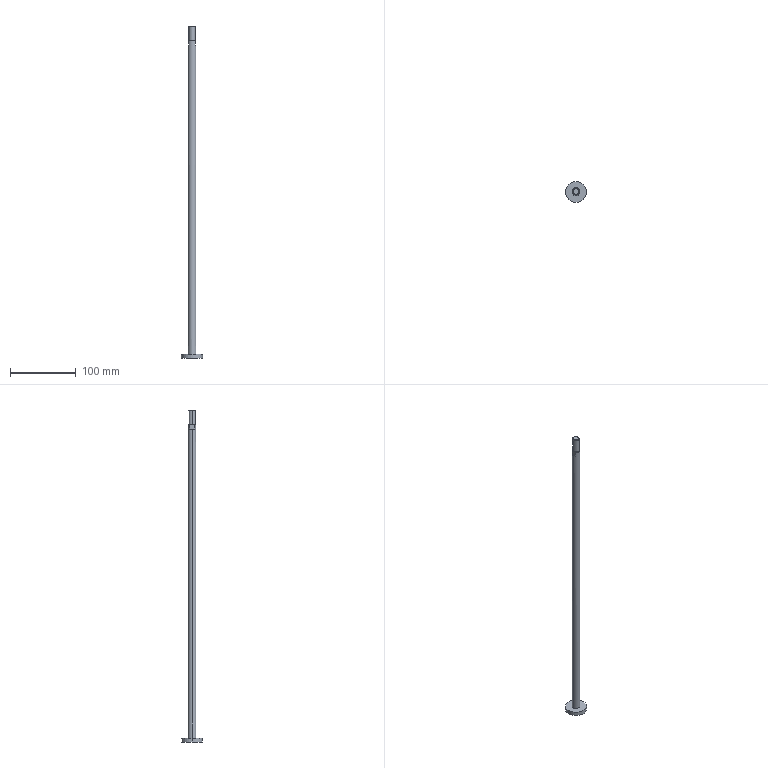Part | STEP file | 1 solid | 17 faces | box 32 x 32 x 503.2 mm | volume 60225 mm3 | plane 9 | cylinder 6 | cone 2 | commonest cylinder face diameters 10 x2 12 x2 32 x2
STEP:
#1=CARTESIAN_POINT('',(0.,0.,0.));
#2=DIRECTION('',(0.,0.,1.));
#3=DIRECTION('',(1.,0.,0.));
#4=AXIS2_PLACEMENT_3D('',#1,#2,#3);
#5=CARTESIAN_POINT('',(5.,0.,26.));
#6=VERTEX_POINT('',#5);
#7=CARTESIAN_POINT('',(-5.,0.,26.));
#8=VERTEX_POINT('',#7);
#9=CARTESIAN_POINT('',(0.,0.,26.));
#10=DIRECTION('',(0.,0.,1.));
#11=DIRECTION('',(1.,0.,0.));
#12=AXIS2_PLACEMENT_3D('',#9,#10,#11);
#13=CIRCLE('',#12,5.);
#14=CARTESIAN_POINT('',(0.,0.,26.));
#15=DIRECTION('',(0.,0.,1.));
#16=DIRECTION('',(1.,0.,0.));
#17=AXIS2_PLACEMENT_3D('',#14,#15,#16);
#18=CYLINDRICAL_SURFACE('',#17,5.);
#19=CARTESIAN_POINT('',(0.,0.));
#20=DIRECTION('',(1.,0.));
#21=VECTOR('',#20,1.);
#22=LINE('',#19,#21);
#23=(GEOMETRIC_REPRESENTATION_CONTEXT(2)PARAMETRIC_REPRESENTATION_CONTEXT()REPRESENTATION_CONTEXT('',''));
#24=DEFINITIONAL_REPRESENTATION('',(#22),#23);
#25=PCURVE('',#18,#24);
#26=CARTESIAN_POINT('',(0.,0.,26.));
#27=DIRECTION('',(0.,0.,-1.));
#28=DIRECTION('',(-1.,0.,0.));
#29=AXIS2_PLACEMENT_3D('',#26,#27,#28);
#30=PLANE('',#29);
#31=CARTESIAN_POINT('',(-5.,0.));
#32=CARTESIAN_POINT('',(-5.,8.66));
#33=CARTESIAN_POINT('',(2.5,4.33));
#34=CARTESIAN_POINT('',(10.,0.));
#35=CARTESIAN_POINT('',(2.5,-4.33));
#36=CARTESIAN_POINT('',(-5.,-8.66));
#37=CARTESIAN_POINT('',(-5.,0.));
#38=(BOUNDED_CURVE()B_SPLINE_CURVE(2,(#31,#32,#33,#34,#35,#36,#37),.UNSPECIFIED.,.T.,.F.)B_SPLINE_CURVE_WITH_KNOTS((1,2,2,2,2,1),(-2.094,0.,2.094,4.189,6.283,8.378),.UNSPECIFIED.)CURVE()GEOMETRIC_REPRESENTATION_ITEM()RATIONAL_B_SPLINE_CURVE((1.,0.5,1.,0.5,1.,0.5,1.))REPRESENTATION_ITEM(''));
#39=(GEOMETRIC_REPRESENTATION_CONTEXT(2)PARAMETRIC_REPRESENTATION_CONTEXT()REPRESENTATION_CONTEXT('',''));
#40=DEFINITIONAL_REPRESENTATION('',(#38),#39);
#41=PCURVE('',#30,#40);
#42=SURFACE_CURVE('',#13,(#25,#41),.PCURVE_S1.);
#43=EDGE_CURVE('',#6,#8,#42,.T.);
#44=ORIENTED_EDGE('',*,*,#43,.T.);
#45=CARTESIAN_POINT('',(-5.,0.,47.233));
#46=VERTEX_POINT('',#45);
#47=CARTESIAN_POINT('',(-5.,0.,26.));
#48=DIRECTION('',(0.,0.,1.));
#49=VECTOR('',#48,1.);
#50=LINE('',#47,#49);
#51=CARTESIAN_POINT('',(3.142,0.));
#52=DIRECTION('',(0.,1.));
#53=VECTOR('',#52,1.);
#54=LINE('',#51,#53);
#55=(GEOMETRIC_REPRESENTATION_CONTEXT(2)PARAMETRIC_REPRESENTATION_CONTEXT()REPRESENTATION_CONTEXT('',''));
#56=DEFINITIONAL_REPRESENTATION('',(#54),#55);
#57=PCURVE('',#18,#56);
#58=CARTESIAN_POINT('',(0.,0.,26.));
#59=DIRECTION('',(0.,0.,1.));
#60=DIRECTION('',(1.,0.,0.));
#61=AXIS2_PLACEMENT_3D('',#58,#59,#60);
#62=CYLINDRICAL_SURFACE('',#61,5.);
#63=CARTESIAN_POINT('',(3.142,0.));
#64=DIRECTION('',(0.,1.));
#65=VECTOR('',#64,1.);
#66=LINE('',#63,#65);
#67=(GEOMETRIC_REPRESENTATION_CONTEXT(2)PARAMETRIC_REPRESENTATION_CONTEXT()REPRESENTATION_CONTEXT('',''));
#68=DEFINITIONAL_REPRESENTATION('',(#66),#67);
#69=PCURVE('',#62,#68);
#70=SURFACE_CURVE('',#50,(#57,#69),.PCURVE_S1.);
#71=EDGE_CURVE('',#8,#46,#70,.T.);
#72=ORIENTED_EDGE('',*,*,#71,.T.);
#73=CARTESIAN_POINT('',(5.,0.,47.233));
#74=VERTEX_POINT('',#73);
#75=CARTESIAN_POINT('',(0.,0.,47.233));
#76=DIRECTION('',(0.,0.,1.));
#77=DIRECTION('',(1.,0.,0.));
#78=AXIS2_PLACEMENT_3D('',#75,#76,#77);
#79=CIRCLE('',#78,5.);
#80=CARTESIAN_POINT('',(0.,21.233));
#81=DIRECTION('',(1.,0.));
#82=VECTOR('',#81,1.);
#83=LINE('',#80,#82);
#84=(GEOMETRIC_REPRESENTATION_CONTEXT(2)PARAMETRIC_REPRESENTATION_CONTEXT()REPRESENTATION_CONTEXT('',''));
#85=DEFINITIONAL_REPRESENTATION('',(#83),#84);
#86=PCURVE('',#18,#85);
#87=CARTESIAN_POINT('',(0.,0.,47.233));
#88=DIRECTION('',(0.,0.,-1.));
#89=DIRECTION('',(-1.,0.,0.));
#90=AXIS2_PLACEMENT_3D('',#87,#88,#89);
#91=CONICAL_SURFACE('',#90,5.,0.7854);
#92=CARTESIAN_POINT('',(3.142,0.));
#93=DIRECTION('',(-1.,0.));
#94=VECTOR('',#93,1.);
#95=LINE('',#92,#94);
#96=(GEOMETRIC_REPRESENTATION_CONTEXT(2)PARAMETRIC_REPRESENTATION_CONTEXT()REPRESENTATION_CONTEXT('',''));
#97=DEFINITIONAL_REPRESENTATION('',(#95),#96);
#98=PCURVE('',#91,#97);
#99=SURFACE_CURVE('',#79,(#86,#98),.PCURVE_S1.);
#100=EDGE_CURVE('',#74,#46,#99,.T.);
#101=ORIENTED_EDGE('',*,*,#100,.F.);
#102=CARTESIAN_POINT('',(5.,0.,26.));
#103=DIRECTION('',(0.,0.,1.));
#104=VECTOR('',#103,1.);
#105=LINE('',#102,#104);
#106=CARTESIAN_POINT('',(0.,0.));
#107=DIRECTION('',(0.,1.));
#108=VECTOR('',#107,1.);
#109=LINE('',#106,#108);
#110=(GEOMETRIC_REPRESENTATION_CONTEXT(2)PARAMETRIC_REPRESENTATION_CONTEXT()REPRESENTATION_CONTEXT('',''));
#111=DEFINITIONAL_REPRESENTATION('',(#109),#110);
#112=PCURVE('',#18,#111);
#113=CARTESIAN_POINT('',(6.283,0.));
#114=DIRECTION('',(0.,1.));
#115=VECTOR('',#114,1.);
#116=LINE('',#113,#115);
#117=(GEOMETRIC_REPRESENTATION_CONTEXT(2)PARAMETRIC_REPRESENTATION_CONTEXT()REPRESENTATION_CONTEXT('',''));
#118=DEFINITIONAL_REPRESENTATION('',(#116),#117);
#119=PCURVE('',#62,#118);
#120=SURFACE_CURVE('',#105,(#112,#119),.PCURVE_S1.);
#121=EDGE_CURVE('',#6,#74,#120,.T.);
#122=ORIENTED_EDGE('',*,*,#121,.F.);
#123=EDGE_LOOP('',(#44,#72,#101,#122));
#124=FACE_BOUND('',#123,.T.);
#125=ADVANCED_FACE('',(#124),#18,.T.);
#126=CARTESIAN_POINT('',(4.233,0.,48.));
#127=VERTEX_POINT('',#126);
#128=CARTESIAN_POINT('',(-4.233,0.,48.));
#129=VERTEX_POINT('',#128);
#130=CARTESIAN_POINT('',(0.,0.,48.));
#131=DIRECTION('',(0.,0.,1.));
#132=DIRECTION('',(1.,0.,0.));
#133=AXIS2_PLACEMENT_3D('',#130,#131,#132);
#134=CIRCLE('',#133,4.233);
#135=CARTESIAN_POINT('',(3.142,-0.767));
#136=DIRECTION('',(-1.,0.));
#137=VECTOR('',#136,1.);
#138=LINE('',#135,#137);
#139=(GEOMETRIC_REPRESENTATION_CONTEXT(2)PARAMETRIC_REPRESENTATION_CONTEXT()REPRESENTATION_CONTEXT('',''));
#140=DEFINITIONAL_REPRESENTATION('',(#138),#139);
#141=PCURVE('',#91,#140);
#142=CARTESIAN_POINT('',(0.,0.,48.));
#143=DIRECTION('',(0.,0.,-1.));
#144=DIRECTION('',(-1.,0.,0.));
#145=AXIS2_PLACEMENT_3D('',#142,#143,#144);
#146=PLANE('',#145);
#147=CARTESIAN_POINT('',(-4.233,0.));
#148=CARTESIAN_POINT('',(-4.233,7.332));
#149=CARTESIAN_POINT('',(2.116,3.666));
#150=CARTESIAN_POINT('',(8.466,0.));
#151=CARTESIAN_POINT('',(2.116,-3.666));
#152=CARTESIAN_POINT('',(-4.233,-7.332));
#153=CARTESIAN_POINT('',(-4.233,0.));
#154=(BOUNDED_CURVE()B_SPLINE_CURVE(2,(#147,#148,#149,#150,#151,#152,#153),.UNSPECIFIED.,.T.,.F.)B_SPLINE_CURVE_WITH_KNOTS((1,2,2,2,2,1),(-2.094,0.,2.094,4.189,6.283,8.378),.UNSPECIFIED.)CURVE()GEOMETRIC_REPRESENTATION_ITEM()RATIONAL_B_SPLINE_CURVE((1.,0.5,1.,0.5,1.,0.5,1.))REPRESENTATION_ITEM(''));
#155=(GEOMETRIC_REPRESENTATION_CONTEXT(2)PARAMETRIC_REPRESENTATION_CONTEXT()REPRESENTATION_CONTEXT('',''));
#156=DEFINITIONAL_REPRESENTATION('',(#154),#155);
#157=PCURVE('',#146,#156);
#158=SURFACE_CURVE('',#134,(#141,#157),.PCURVE_S1.);
#159=EDGE_CURVE('',#127,#129,#158,.T.);
#160=ORIENTED_EDGE('',*,*,#159,.F.);
#161=CARTESIAN_POINT('',(5.,0.,47.233));
#162=DIRECTION('',(0.7071,0.,-0.7071));
#163=VECTOR('',#162,1.);
#164=LINE('',#161,#163);
#165=CARTESIAN_POINT('',(3.142,0.));
#166=DIRECTION('',(0.,1.));
#167=VECTOR('',#166,1.);
#168=LINE('',#165,#167);
#169=(GEOMETRIC_REPRESENTATION_CONTEXT(2)PARAMETRIC_REPRESENTATION_CONTEXT()REPRESENTATION_CONTEXT('',''));
#170=DEFINITIONAL_REPRESENTATION('',(#168),#169);
#171=PCURVE('',#91,#170);
#172=CARTESIAN_POINT('',(0.,0.,47.233));
#173=DIRECTION('',(0.,0.,-1.));
#174=DIRECTION('',(-1.,0.,0.));
#175=AXIS2_PLACEMENT_3D('',#172,#173,#174);
#176=CONICAL_SURFACE('',#175,5.,0.7854);
#177=CARTESIAN_POINT('',(3.142,0.));
#178=DIRECTION('',(0.,1.));
#179=VECTOR('',#178,1.);
#180=LINE('',#177,#179);
#181=(GEOMETRIC_REPRESENTATION_CONTEXT(2)PARAMETRIC_REPRESENTATION_CONTEXT()REPRESENTATION_CONTEXT('',''));
#182=DEFINITIONAL_REPRESENTATION('',(#180),#181);
#183=PCURVE('',#176,#182);
#184=SURFACE_CURVE('',#164,(#171,#183),.PCURVE_S1.);
#185=EDGE_CURVE('',#127,#74,#184,.T.);
#186=ORIENTED_EDGE('',*,*,#185,.T.);
#187=ORIENTED_EDGE('',*,*,#100,.T.);
#188=CARTESIAN_POINT('',(-5.,0.,47.233));
#189=DIRECTION('',(-0.7071,0.,-0.7071));
#190=VECTOR('',#189,1.);
#191=LINE('',#188,#190);
#192=CARTESIAN_POINT('',(0.,0.));
#193=DIRECTION('',(0.,1.));
#194=VECTOR('',#193,1.);
#195=LINE('',#192,#194);
#196=(GEOMETRIC_REPRESENTATION_CONTEXT(2)PARAMETRIC_REPRESENTATION_CONTEXT()REPRESENTATION_CONTEXT('',''));
#197=DEFINITIONAL_REPRESENTATION('',(#195),#196);
#198=PCURVE('',#91,#197);
#199=CARTESIAN_POINT('',(6.283,0.));
#200=DIRECTION('',(0.,1.));
#201=VECTOR('',#200,1.);
#202=LINE('',#199,#201);
#203=(GEOMETRIC_REPRESENTATION_CONTEXT(2)PARAMETRIC_REPRESENTATION_CONTEXT()REPRESENTATION_CONTEXT('',''));
#204=DEFINITIONAL_REPRESENTATION('',(#202),#203);
#205=PCURVE('',#176,#204);
#206=SURFACE_CURVE('',#191,(#198,#205),.PCURVE_S1.);
#207=EDGE_CURVE('',#129,#46,#206,.T.);
#208=ORIENTED_EDGE('',*,*,#207,.F.);
#209=EDGE_LOOP('',(#160,#186,#187,#208));
#210=FACE_BOUND('',#209,.T.);
#211=ADVANCED_FACE('',(#210),#91,.T.);
#212=CARTESIAN_POINT('',(16.,0.,-455.2));
#213=VERTEX_POINT('',#212);
#214=CARTESIAN_POINT('',(-16.,0.,-455.2));
#215=VERTEX_POINT('',#214);
#216=CARTESIAN_POINT('',(0.,0.,-455.2));
#217=DIRECTION('',(0.,0.,1.));
#218=DIRECTION('',(1.,0.,0.));
#219=AXIS2_PLACEMENT_3D('',#216,#217,#218);
#220=CIRCLE('',#219,16.);
#221=CARTESIAN_POINT('',(0.,0.,-455.2));
#222=DIRECTION('',(0.,0.,1.));
#223=DIRECTION('',(1.,0.,0.));
#224=AXIS2_PLACEMENT_3D('',#221,#222,#223);
#225=CYLINDRICAL_SURFACE('',#224,16.);
#226=CARTESIAN_POINT('',(0.,0.));
#227=DIRECTION('',(1.,0.));
#228=VECTOR('',#227,1.);
#229=LINE('',#226,#228);
#230=(GEOMETRIC_REPRESENTATION_CONTEXT(2)PARAMETRIC_REPRESENTATION_CONTEXT()REPRESENTATION_CONTEXT('',''));
#231=DEFINITIONAL_REPRESENTATION('',(#229),#230);
#232=PCURVE('',#225,#231);
#233=CARTESIAN_POINT('',(0.,16.,-455.2));
#234=DIRECTION('',(0.,0.,1.));
#235=DIRECTION('',(1.,0.,0.));
#236=AXIS2_PLACEMENT_3D('',#233,#234,#235);
#237=PLANE('',#236);
#238=CARTESIAN_POINT('',(0.,-16.));
#239=DIRECTION('',(1.,0.));
#240=AXIS2_PLACEMENT_2D('',#238,#239);
#241=CIRCLE('',#240,16.);
#242=(GEOMETRIC_REPRESENTATION_CONTEXT(2)PARAMETRIC_REPRESENTATION_CONTEXT()REPRESENTATION_CONTEXT('',''));
#243=DEFINITIONAL_REPRESENTATION('',(#241),#242);
#244=PCURVE('',#237,#243);
#245=SURFACE_CURVE('',#220,(#232,#244),.PCURVE_S1.);
#246=EDGE_CURVE('',#213,#215,#245,.T.);
#247=ORIENTED_EDGE('',*,*,#246,.T.);
#248=CARTESIAN_POINT('',(-16.,0.,-449.2));
#249=VERTEX_POINT('',#248);
#250=CARTESIAN_POINT('',(-16.,0.,-455.2));
#251=DIRECTION('',(0.,0.,1.));
#252=VECTOR('',#251,1.);
#253=LINE('',#250,#252);
#254=CARTESIAN_POINT('',(3.142,0.));
#255=DIRECTION('',(0.,1.));
#256=VECTOR('',#255,1.);
#257=LINE('',#254,#256);
#258=(GEOMETRIC_REPRESENTATION_CONTEXT(2)PARAMETRIC_REPRESENTATION_CONTEXT()REPRESENTATION_CONTEXT('',''));
#259=DEFINITIONAL_REPRESENTATION('',(#257),#258);
#260=PCURVE('',#225,#259);
#261=CARTESIAN_POINT('',(0.,0.,-455.2));
#262=DIRECTION('',(0.,0.,1.));
#263=DIRECTION('',(1.,0.,0.));
#264=AXIS2_PLACEMENT_3D('',#261,#262,#263);
#265=CYLINDRICAL_SURFACE('',#264,16.);
#266=CARTESIAN_POINT('',(3.142,0.));
#267=DIRECTION('',(0.,1.));
#268=VECTOR('',#267,1.);
#269=LINE('',#266,#268);
#270=(GEOMETRIC_REPRESENTATION_CONTEXT(2)PARAMETRIC_REPRESENTATION_CONTEXT()REPRESENTATION_CONTEXT('',''));
#271=DEFINITIONAL_REPRESENTATION('',(#269),#270);
#272=PCURVE('',#265,#271);
#273=SURFACE_CURVE('',#253,(#260,#272),.PCURVE_S1.);
#274=EDGE_CURVE('',#215,#249,#273,.T.);
#275=ORIENTED_EDGE('',*,*,#274,.T.);
#276=CARTESIAN_POINT('',(16.,0.,-449.2));
#277=VERTEX_POINT('',#276);
#278=CARTESIAN_POINT('',(0.,0.,-449.2));
#279=DIRECTION('',(0.,0.,1.));
#280=DIRECTION('',(1.,0.,0.));
#281=AXIS2_PLACEMENT_3D('',#278,#279,#280);
#282=CIRCLE('',#281,16.);
#283=CARTESIAN_POINT('',(0.,6.));
#284=DIRECTION('',(1.,0.));
#285=VECTOR('',#284,1.);
#286=LINE('',#283,#285);
#287=(GEOMETRIC_REPRESENTATION_CONTEXT(2)PARAMETRIC_REPRESENTATION_CONTEXT()REPRESENTATION_CONTEXT('',''));
#288=DEFINITIONAL_REPRESENTATION('',(#286),#287);
#289=PCURVE('',#225,#288);
#290=CARTESIAN_POINT('',(0.,6.,-449.2));
#291=DIRECTION('',(0.,0.,-1.));
#292=DIRECTION('',(-1.,0.,0.));
#293=AXIS2_PLACEMENT_3D('',#290,#291,#292);
#294=PLANE('',#293);
#295=CARTESIAN_POINT('',(-16.,-6.));
#296=CARTESIAN_POINT('',(-16.,21.713));
#297=CARTESIAN_POINT('',(8.,7.856));
#298=CARTESIAN_POINT('',(32.,-6.));
#299=CARTESIAN_POINT('',(8.,-19.856));
#300=CARTESIAN_POINT('',(-16.,-33.713));
#301=CARTESIAN_POINT('',(-16.,-6.));
#302=(BOUNDED_CURVE()B_SPLINE_CURVE(2,(#295,#296,#297,#298,#299,#300,#301),.UNSPECIFIED.,.T.,.F.)B_SPLINE_CURVE_WITH_KNOTS((1,2,2,2,2,1),(-2.094,0.,2.094,4.189,6.283,8.378),.UNSPECIFIED.)CURVE()GEOMETRIC_REPRESENTATION_ITEM()RATIONAL_B_SPLINE_CURVE((1.,0.5,1.,0.5,1.,0.5,1.))REPRESENTATION_ITEM(''));
#303=(GEOMETRIC_REPRESENTATION_CONTEXT(2)PARAMETRIC_REPRESENTATION_CONTEXT()REPRESENTATION_CONTEXT('',''));
#304=DEFINITIONAL_REPRESENTATION('',(#302),#303);
#305=PCURVE('',#294,#304);
#306=SURFACE_CURVE('',#282,(#289,#305),.PCURVE_S1.);
#307=EDGE_CURVE('',#277,#249,#306,.T.);
#308=ORIENTED_EDGE('',*,*,#307,.F.);
#309=CARTESIAN_POINT('',(16.,0.,-455.2));
#310=DIRECTION('',(0.,0.,1.));
#311=VECTOR('',#310,1.);
#312=LINE('',#309,#311);
#313=CARTESIAN_POINT('',(0.,0.));
#314=DIRECTION('',(0.,1.));
#315=VECTOR('',#314,1.);
#316=LINE('',#313,#315);
#317=(GEOMETRIC_REPRESENTATION_CONTEXT(2)PARAMETRIC_REPRESENTATION_CONTEXT()REPRESENTATION_CONTEXT('',''));
#318=DEFINITIONAL_REPRESENTATION('',(#316),#317);
#319=PCURVE('',#225,#318);
#320=CARTESIAN_POINT('',(6.283,0.));
#321=DIRECTION('',(0.,1.));
#322=VECTOR('',#321,1.);
#323=LINE('',#320,#322);
#324=(GEOMETRIC_REPRESENTATION_CONTEXT(2)PARAMETRIC_REPRESENTATION_CONTEXT()REPRESENTATION_CONTEXT('',''));
#325=DEFINITIONAL_REPRESENTATION('',(#323),#324);
#326=PCURVE('',#265,#325);
#327=SURFACE_CURVE('',#312,(#319,#326),.PCURVE_S1.);
#328=EDGE_CURVE('',#213,#277,#327,.T.);
#329=ORIENTED_EDGE('',*,*,#328,.F.);
#330=EDGE_LOOP('',(#247,#275,#308,#329));
#331=FACE_BOUND('',#330,.T.);
#332=ADVANCED_FACE('',(#331),#225,.T.);
#333=CARTESIAN_POINT('',(6.,0.,-449.2));
#334=VERTEX_POINT('',#333);
#335=CARTESIAN_POINT('',(-6.,0.,-449.2));
#336=VERTEX_POINT('',#335);
#337=CARTESIAN_POINT('',(0.,0.,-449.2));
#338=DIRECTION('',(0.,0.,1.));
#339=DIRECTION('',(1.,0.,0.));
#340=AXIS2_PLACEMENT_3D('',#337,#338,#339);
#341=CIRCLE('',#340,6.);
#342=CARTESIAN_POINT('',(0.,0.,-455.2));
#343=DIRECTION('',(0.,0.,1.));
#344=DIRECTION('',(1.,0.,0.));
#345=AXIS2_PLACEMENT_3D('',#342,#343,#344);
#346=CYLINDRICAL_SURFACE('',#345,6.);
#347=CARTESIAN_POINT('',(0.,6.));
#348=DIRECTION('',(1.,0.));
#349=VECTOR('',#348,1.);
#350=LINE('',#347,#349);
#351=(GEOMETRIC_REPRESENTATION_CONTEXT(2)PARAMETRIC_REPRESENTATION_CONTEXT()REPRESENTATION_CONTEXT('',''));
#352=DEFINITIONAL_REPRESENTATION('',(#350),#351);
#353=PCURVE('',#346,#352);
#354=CARTESIAN_POINT('',(-6.,-6.));
#355=CARTESIAN_POINT('',(-6.,4.392));
#356=CARTESIAN_POINT('',(3.,-0.8038));
#357=CARTESIAN_POINT('',(12.,-6.));
#358=CARTESIAN_POINT('',(3.,-11.196));
#359=CARTESIAN_POINT('',(-6.,-16.392));
#360=CARTESIAN_POINT('',(-6.,-6.));
#361=(BOUNDED_CURVE()B_SPLINE_CURVE(2,(#354,#355,#356,#357,#358,#359,#360),.UNSPECIFIED.,.T.,.F.)B_SPLINE_CURVE_WITH_KNOTS((1,2,2,2,2,1),(-2.094,0.,2.094,4.189,6.283,8.378),.UNSPECIFIED.)CURVE()GEOMETRIC_REPRESENTATION_ITEM()RATIONAL_B_SPLINE_CURVE((1.,0.5,1.,0.5,1.,0.5,1.))REPRESENTATION_ITEM(''));
#362=(GEOMETRIC_REPRESENTATION_CONTEXT(2)PARAMETRIC_REPRESENTATION_CONTEXT()REPRESENTATION_CONTEXT('',''));
#363=DEFINITIONAL_REPRESENTATION('',(#361),#362);
#364=PCURVE('',#294,#363);
#365=SURFACE_CURVE('',#341,(#353,#364),.PCURVE_S1.);
#366=EDGE_CURVE('',#334,#336,#365,.T.);
#367=ORIENTED_EDGE('',*,*,#366,.T.);
#368=CARTESIAN_POINT('',(-6.,0.,19.));
#369=VERTEX_POINT('',#368);
#370=CARTESIAN_POINT('',(-6.,0.,-455.2));
#371=DIRECTION('',(0.,0.,1.));
#372=VECTOR('',#371,1.);
#373=LINE('',#370,#372);
#374=CARTESIAN_POINT('',(3.142,0.));
#375=DIRECTION('',(0.,1.));
#376=VECTOR('',#375,1.);
#377=LINE('',#374,#376);
#378=(GEOMETRIC_REPRESENTATION_CONTEXT(2)PARAMETRIC_REPRESENTATION_CONTEXT()REPRESENTATION_CONTEXT('',''));
#379=DEFINITIONAL_REPRESENTATION('',(#377),#378);
#380=PCURVE('',#346,#379);
#381=CARTESIAN_POINT('',(0.,0.,-455.2));
#382=DIRECTION('',(0.,0.,1.));
#383=DIRECTION('',(1.,0.,0.));
#384=AXIS2_PLACEMENT_3D('',#381,#382,#383);
#385=CYLINDRICAL_SURFACE('',#384,6.);
#386=CARTESIAN_POINT('',(3.142,0.));
#387=DIRECTION('',(0.,1.));
#388=VECTOR('',#387,1.);
#389=LINE('',#386,#388);
#390=(GEOMETRIC_REPRESENTATION_CONTEXT(2)PARAMETRIC_REPRESENTATION_CONTEXT()REPRESENTATION_CONTEXT('',''));
#391=DEFINITIONAL_REPRESENTATION('',(#389),#390);
#392=PCURVE('',#385,#391);
#393=SURFACE_CURVE('',#373,(#380,#392),.PCURVE_S1.);
#394=EDGE_CURVE('',#336,#369,#393,.T.);
#395=ORIENTED_EDGE('',*,*,#394,.T.);
#396=CARTESIAN_POINT('',(-5.,3.317,19.));
#397=VERTEX_POINT('',#396);
#398=CARTESIAN_POINT('',(0.,0.,19.));
#399=DIRECTION('',(0.,0.,1.));
#400=DIRECTION('',(1.,0.,0.));
#401=AXIS2_PLACEMENT_3D('',#398,#399,#400);
#402=CIRCLE('',#401,6.);
#403=CARTESIAN_POINT('',(0.,474.2));
#404=DIRECTION('',(1.,0.));
#405=VECTOR('',#404,1.);
#406=LINE('',#403,#405);
#407=(GEOMETRIC_REPRESENTATION_CONTEXT(2)PARAMETRIC_REPRESENTATION_CONTEXT()REPRESENTATION_CONTEXT('',''));
#408=DEFINITIONAL_REPRESENTATION('',(#406),#407);
#409=PCURVE('',#346,#408);
#410=CARTESIAN_POINT('',(0.,0.,19.));
#411=DIRECTION('',(0.,0.,1.));
#412=DIRECTION('',(1.,0.,0.));
#413=AXIS2_PLACEMENT_3D('',#410,#411,#412);
#414=PLANE('',#413);
#415=CARTESIAN_POINT('',(0.,0.));
#416=DIRECTION('',(1.,0.));
#417=AXIS2_PLACEMENT_2D('',#415,#416);
#418=CIRCLE('',#417,6.);
#419=(GEOMETRIC_REPRESENTATION_CONTEXT(2)PARAMETRIC_REPRESENTATION_CONTEXT()REPRESENTATION_CONTEXT('',''));
#420=DEFINITIONAL_REPRESENTATION('',(#418),#419);
#421=PCURVE('',#414,#420);
#422=SURFACE_CURVE('',#402,(#409,#421),.PCURVE_S1.);
#423=EDGE_CURVE('',#397,#369,#422,.T.);
#424=ORIENTED_EDGE('',*,*,#423,.F.);
#425=CARTESIAN_POINT('',(-5.,3.317,26.));
#426=VERTEX_POINT('',#425);
#427=CARTESIAN_POINT('',(-5.,3.317,-455.2));
#428=DIRECTION('',(0.,0.,1.));
#429=VECTOR('',#428,1.);
#430=LINE('',#427,#429);
#431=CARTESIAN_POINT('',(2.556,0.));
#432=DIRECTION('',(0.,1.));
#433=VECTOR('',#432,1.);
#434=LINE('',#431,#433);
#435=(GEOMETRIC_REPRESENTATION_CONTEXT(2)PARAMETRIC_REPRESENTATION_CONTEXT()REPRESENTATION_CONTEXT('',''));
#436=DEFINITIONAL_REPRESENTATION('',(#434),#435);
#437=PCURVE('',#346,#436);
#438=CARTESIAN_POINT('',(-5.,-10.,19.));
#439=DIRECTION('',(1.,0.,0.));
#440=DIRECTION('',(0.,0.,-1.));
#441=AXIS2_PLACEMENT_3D('',#438,#439,#440);
#442=PLANE('',#441);
#443=CARTESIAN_POINT('',(474.2,13.317));
#444=DIRECTION('',(-1.,0.));
#445=VECTOR('',#444,1.);
#446=LINE('',#443,#445);
#447=(GEOMETRIC_REPRESENTATION_CONTEXT(2)PARAMETRIC_REPRESENTATION_CONTEXT()REPRESENTATION_CONTEXT('',''));
#448=DEFINITIONAL_REPRESENTATION('',(#446),#447);
#449=PCURVE('',#442,#448);
#450=SURFACE_CURVE('',#430,(#437,#449),.PCURVE_S1.);
#451=EDGE_CURVE('',#397,#426,#450,.T.);
#452=ORIENTED_EDGE('',*,*,#451,.T.);
#453=CARTESIAN_POINT('',(5.,3.317,26.));
#454=VERTEX_POINT('',#453);
#455=CARTESIAN_POINT('',(0.,0.,26.));
#456=DIRECTION('',(0.,0.,1.));
#457=DIRECTION('',(1.,0.,0.));
#458=AXIS2_PLACEMENT_3D('',#455,#456,#457);
#459=CIRCLE('',#458,6.);
#460=CARTESIAN_POINT('',(0.,481.2));
#461=DIRECTION('',(1.,0.));
#462=VECTOR('',#461,1.);
#463=LINE('',#460,#462);
#464=(GEOMETRIC_REPRESENTATION_CONTEXT(2)PARAMETRIC_REPRESENTATION_CONTEXT()REPRESENTATION_CONTEXT('',''));
#465=DEFINITIONAL_REPRESENTATION('',(#463),#464);
#466=PCURVE('',#346,#465);
#467=CARTESIAN_POINT('',(-6.,0.));
#468=CARTESIAN_POINT('',(-6.,10.392));
#469=CARTESIAN_POINT('',(3.,5.196));
#470=CARTESIAN_POINT('',(12.,0.));
#471=CARTESIAN_POINT('',(3.,-5.196));
#472=CARTESIAN_POINT('',(-6.,-10.392));
#473=CARTESIAN_POINT('',(-6.,0.));
#474=(BOUNDED_CURVE()B_SPLINE_CURVE(2,(#467,#468,#469,#470,#471,#472,#473),.UNSPECIFIED.,.T.,.F.)B_SPLINE_CURVE_WITH_KNOTS((1,2,2,2,2,1),(-2.094,0.,2.094,4.189,6.283,8.378),.UNSPECIFIED.)CURVE()GEOMETRIC_REPRESENTATION_ITEM()RATIONAL_B_SPLINE_CURVE((1.,0.5,1.,0.5,1.,0.5,1.))REPRESENTATION_ITEM(''));
#475=(GEOMETRIC_REPRESENTATION_CONTEXT(2)PARAMETRIC_REPRESENTATION_CONTEXT()REPRESENTATION_CONTEXT('',''));
#476=DEFINITIONAL_REPRESENTATION('',(#474),#475);
#477=PCURVE('',#30,#476);
#478=SURFACE_CURVE('',#459,(#466,#477),.PCURVE_S1.);
#479=EDGE_CURVE('',#454,#426,#478,.T.);
#480=ORIENTED_EDGE('',*,*,#479,.F.);
#481=CARTESIAN_POINT('',(5.,3.317,19.));
#482=VERTEX_POINT('',#481);
#483=CARTESIAN_POINT('',(5.,3.317,-455.2));
#484=DIRECTION('',(0.,0.,-1.));
#485=VECTOR('',#484,1.);
#486=LINE('',#483,#485);
#487=CARTESIAN_POINT('',(0.5857,0.));
#488=DIRECTION('',(0.,-1.));
#489=VECTOR('',#488,1.);
#490=LINE('',#487,#489);
#491=(GEOMETRIC_REPRESENTATION_CONTEXT(2)PARAMETRIC_REPRESENTATION_CONTEXT()REPRESENTATION_CONTEXT('',''));
#492=DEFINITIONAL_REPRESENTATION('',(#490),#491);
#493=PCURVE('',#346,#492);
#494=CARTESIAN_POINT('',(5.,10.,19.));
#495=DIRECTION('',(-1.,0.,0.));
#496=DIRECTION('',(0.,0.,1.));
#497=AXIS2_PLACEMENT_3D('',#494,#495,#496);
#498=PLANE('',#497);
#499=CARTESIAN_POINT('',(-474.2,-6.683));
#500=DIRECTION('',(-1.,0.));
#501=VECTOR('',#500,1.);
#502=LINE('',#499,#501);
#503=(GEOMETRIC_REPRESENTATION_CONTEXT(2)PARAMETRIC_REPRESENTATION_CONTEXT()REPRESENTATION_CONTEXT('',''));
#504=DEFINITIONAL_REPRESENTATION('',(#502),#503);
#505=PCURVE('',#498,#504);
#506=SURFACE_CURVE('',#486,(#493,#505),.PCURVE_S1.);
#507=EDGE_CURVE('',#454,#482,#506,.T.);
#508=ORIENTED_EDGE('',*,*,#507,.T.);
#509=CARTESIAN_POINT('',(6.,0.,19.));
#510=VERTEX_POINT('',#509);
#511=CARTESIAN_POINT('',(0.,0.,19.));
#512=DIRECTION('',(0.,0.,1.));
#513=DIRECTION('',(1.,0.,0.));
#514=AXIS2_PLACEMENT_3D('',#511,#512,#513);
#515=CIRCLE('',#514,6.);
#516=CARTESIAN_POINT('',(0.,474.2));
#517=DIRECTION('',(1.,0.));
#518=VECTOR('',#517,1.);
#519=LINE('',#516,#518);
#520=(GEOMETRIC_REPRESENTATION_CONTEXT(2)PARAMETRIC_REPRESENTATION_CONTEXT()REPRESENTATION_CONTEXT('',''));
#521=DEFINITIONAL_REPRESENTATION('',(#519),#520);
#522=PCURVE('',#346,#521);
#523=CARTESIAN_POINT('',(0.,0.,19.));
#524=DIRECTION('',(0.,0.,1.));
#525=DIRECTION('',(1.,0.,0.));
#526=AXIS2_PLACEMENT_3D('',#523,#524,#525);
#527=PLANE('',#526);
#528=CARTESIAN_POINT('',(0.,0.));
#529=DIRECTION('',(1.,0.));
#530=AXIS2_PLACEMENT_2D('',#528,#529);
#531=CIRCLE('',#530,6.);
#532=(GEOMETRIC_REPRESENTATION_CONTEXT(2)PARAMETRIC_REPRESENTATION_CONTEXT()REPRESENTATION_CONTEXT('',''));
#533=DEFINITIONAL_REPRESENTATION('',(#531),#532);
#534=PCURVE('',#527,#533);
#535=SURFACE_CURVE('',#515,(#522,#534),.PCURVE_S1.);
#536=EDGE_CURVE('',#510,#482,#535,.T.);
#537=ORIENTED_EDGE('',*,*,#536,.F.);
#538=CARTESIAN_POINT('',(6.,0.,-455.2));
#539=DIRECTION('',(0.,0.,1.));
#540=VECTOR('',#539,1.);
#541=LINE('',#538,#540);
#542=CARTESIAN_POINT('',(0.,0.));
#543=DIRECTION('',(0.,1.));
#544=VECTOR('',#543,1.);
#545=LINE('',#542,#544);
#546=(GEOMETRIC_REPRESENTATION_CONTEXT(2)PARAMETRIC_REPRESENTATION_CONTEXT()REPRESENTATION_CONTEXT('',''));
#547=DEFINITIONAL_REPRESENTATION('',(#545),#546);
#548=PCURVE('',#346,#547);
#549=CARTESIAN_POINT('',(6.283,0.));
#550=DIRECTION('',(0.,1.));
#551=VECTOR('',#550,1.);
#552=LINE('',#549,#551);
#553=(GEOMETRIC_REPRESENTATION_CONTEXT(2)PARAMETRIC_REPRESENTATION_CONTEXT()REPRESENTATION_CONTEXT('',''));
#554=DEFINITIONAL_REPRESENTATION('',(#552),#553);
#555=PCURVE('',#385,#554);
#556=SURFACE_CURVE('',#541,(#548,#555),.PCURVE_S1.);
#557=EDGE_CURVE('',#334,#510,#556,.T.);
#558=ORIENTED_EDGE('',*,*,#557,.F.);
#559=EDGE_LOOP('',(#367,#395,#424,#452,#480,#508,#537,#558));
#560=FACE_BOUND('',#559,.T.);
#561=ADVANCED_FACE('',(#560),#346,.T.);
#562=ORIENTED_EDGE('',*,*,#43,.F.);
#563=CARTESIAN_POINT('',(5.,10.,26.));
#564=DIRECTION('',(0.,-1.,0.));
#565=VECTOR('',#564,1.);
#566=LINE('',#563,#565);
#567=CARTESIAN_POINT('',(-5.,10.));
#568=DIRECTION('',(0.,-1.));
#569=VECTOR('',#568,1.);
#570=LINE('',#567,#569);
#571=(GEOMETRIC_REPRESENTATION_CONTEXT(2)PARAMETRIC_REPRESENTATION_CONTEXT()REPRESENTATION_CONTEXT('',''));
#572=DEFINITIONAL_REPRESENTATION('',(#570),#571);
#573=PCURVE('',#30,#572);
#574=CARTESIAN_POINT('',(7.,0.));
#575=DIRECTION('',(0.,-1.));
#576=VECTOR('',#575,1.);
#577=LINE('',#574,#576);
#578=(GEOMETRIC_REPRESENTATION_CONTEXT(2)PARAMETRIC_REPRESENTATION_CONTEXT()REPRESENTATION_CONTEXT('',''));
#579=DEFINITIONAL_REPRESENTATION('',(#577),#578);
#580=PCURVE('',#498,#579);
#581=SURFACE_CURVE('',#566,(#573,#580),.PCURVE_S1.);
#582=EDGE_CURVE('',#454,#6,#581,.T.);
#583=ORIENTED_EDGE('',*,*,#582,.F.);
#584=ORIENTED_EDGE('',*,*,#479,.T.);
#585=CARTESIAN_POINT('',(-5.,-10.,26.));
#586=DIRECTION('',(0.,1.,0.));
#587=VECTOR('',#586,1.);
#588=LINE('',#585,#587);
#589=CARTESIAN_POINT('',(5.,-10.));
#590=DIRECTION('',(0.,1.));
#591=VECTOR('',#590,1.);
#592=LINE('',#589,#591);
#593=(GEOMETRIC_REPRESENTATION_CONTEXT(2)PARAMETRIC_REPRESENTATION_CONTEXT()REPRESENTATION_CONTEXT('',''));
#594=DEFINITIONAL_REPRESENTATION('',(#592),#593);
#595=PCURVE('',#30,#594);
#596=CARTESIAN_POINT('',(-7.,0.));
#597=DIRECTION('',(0.,1.));
#598=VECTOR('',#597,1.);
#599=LINE('',#596,#598);
#600=(GEOMETRIC_REPRESENTATION_CONTEXT(2)PARAMETRIC_REPRESENTATION_CONTEXT()REPRESENTATION_CONTEXT('',''));
#601=DEFINITIONAL_REPRESENTATION('',(#599),#600);
#602=PCURVE('',#442,#601);
#603=SURFACE_CURVE('',#588,(#595,#602),.PCURVE_S1.);
#604=EDGE_CURVE('',#8,#426,#603,.T.);
#605=ORIENTED_EDGE('',*,*,#604,.F.);
#606=EDGE_LOOP('',(#562,#583,#584,#605));
#607=FACE_BOUND('',#606,.T.);
#608=ADVANCED_FACE('',(#607),#30,.F.);
#609=CARTESIAN_POINT('',(0.,0.,26.));
#610=DIRECTION('',(0.,0.,1.));
#611=DIRECTION('',(1.,0.,0.));
#612=AXIS2_PLACEMENT_3D('',#609,#610,#611);
#613=CIRCLE('',#612,5.);
#614=CARTESIAN_POINT('',(0.,0.,26.));
#615=DIRECTION('',(0.,0.,-1.));
#616=DIRECTION('',(-1.,0.,0.));
#617=AXIS2_PLACEMENT_3D('',#614,#615,#616);
#618=PLANE('',#617);
#619=CARTESIAN_POINT('',(-5.,0.));
#620=CARTESIAN_POINT('',(-5.,8.66));
#621=CARTESIAN_POINT('',(2.5,4.33));
#622=CARTESIAN_POINT('',(10.,0.));
#623=CARTESIAN_POINT('',(2.5,-4.33));
#624=CARTESIAN_POINT('',(-5.,-8.66));
#625=CARTESIAN_POINT('',(-5.,0.));
#626=(BOUNDED_CURVE()B_SPLINE_CURVE(2,(#619,#620,#621,#622,#623,#624,#625),.UNSPECIFIED.,.T.,.F.)B_SPLINE_CURVE_WITH_KNOTS((1,2,2,2,2,1),(-2.094,0.,2.094,4.189,6.283,8.378),.UNSPECIFIED.)CURVE()GEOMETRIC_REPRESENTATION_ITEM()RATIONAL_B_SPLINE_CURVE((1.,0.5,1.,0.5,1.,0.5,1.))REPRESENTATION_ITEM(''));
#627=(GEOMETRIC_REPRESENTATION_CONTEXT(2)PARAMETRIC_REPRESENTATION_CONTEXT()REPRESENTATION_CONTEXT('',''));
#628=DEFINITIONAL_REPRESENTATION('',(#626),#627);
#629=PCURVE('',#618,#628);
#630=CARTESIAN_POINT('',(0.,0.));
#631=DIRECTION('',(1.,0.));
#632=VECTOR('',#631,1.);
#633=LINE('',#630,#632);
#634=(GEOMETRIC_REPRESENTATION_CONTEXT(2)PARAMETRIC_REPRESENTATION_CONTEXT()REPRESENTATION_CONTEXT('',''));
#635=DEFINITIONAL_REPRESENTATION('',(#633),#634);
#636=PCURVE('',#62,#635);
#637=SURFACE_CURVE('',#613,(#629,#636),.PCURVE_S1.);
#638=EDGE_CURVE('',#8,#6,#637,.T.);
#639=ORIENTED_EDGE('',*,*,#638,.F.);
#640=CARTESIAN_POINT('',(-5.,-3.317,26.));
#641=VERTEX_POINT('',#640);
#642=CARTESIAN_POINT('',(-5.,-10.,26.));
#643=DIRECTION('',(0.,1.,0.));
#644=VECTOR('',#643,1.);
#645=LINE('',#642,#644);
#646=CARTESIAN_POINT('',(5.,-10.));
#647=DIRECTION('',(0.,1.));
#648=VECTOR('',#647,1.);
#649=LINE('',#646,#648);
#650=(GEOMETRIC_REPRESENTATION_CONTEXT(2)PARAMETRIC_REPRESENTATION_CONTEXT()REPRESENTATION_CONTEXT('',''));
#651=DEFINITIONAL_REPRESENTATION('',(#649),#650);
#652=PCURVE('',#618,#651);
#653=CARTESIAN_POINT('',(-7.,0.));
#654=DIRECTION('',(0.,1.));
#655=VECTOR('',#654,1.);
#656=LINE('',#653,#655);
#657=(GEOMETRIC_REPRESENTATION_CONTEXT(2)PARAMETRIC_REPRESENTATION_CONTEXT()REPRESENTATION_CONTEXT('',''));
#658=DEFINITIONAL_REPRESENTATION('',(#656),#657);
#659=PCURVE('',#442,#658);
#660=SURFACE_CURVE('',#645,(#652,#659),.PCURVE_S1.);
#661=EDGE_CURVE('',#641,#8,#660,.T.);
#662=ORIENTED_EDGE('',*,*,#661,.F.);
#663=CARTESIAN_POINT('',(5.,-3.317,26.));
#664=VERTEX_POINT('',#663);
#665=CARTESIAN_POINT('',(0.,0.,26.));
#666=DIRECTION('',(0.,0.,1.));
#667=DIRECTION('',(1.,0.,0.));
#668=AXIS2_PLACEMENT_3D('',#665,#666,#667);
#669=CIRCLE('',#668,6.);
#670=CARTESIAN_POINT('',(-6.,0.));
#671=CARTESIAN_POINT('',(-6.,10.392));
#672=CARTESIAN_POINT('',(3.,5.196));
#673=CARTESIAN_POINT('',(12.,0.));
#674=CARTESIAN_POINT('',(3.,-5.196));
#675=CARTESIAN_POINT('',(-6.,-10.392));
#676=CARTESIAN_POINT('',(-6.,0.));
#677=(BOUNDED_CURVE()B_SPLINE_CURVE(2,(#670,#671,#672,#673,#674,#675,#676),.UNSPECIFIED.,.T.,.F.)B_SPLINE_CURVE_WITH_KNOTS((1,2,2,2,2,1),(-2.094,0.,2.094,4.189,6.283,8.378),.UNSPECIFIED.)CURVE()GEOMETRIC_REPRESENTATION_ITEM()RATIONAL_B_SPLINE_CURVE((1.,0.5,1.,0.5,1.,0.5,1.))REPRESENTATION_ITEM(''));
#678=(GEOMETRIC_REPRESENTATION_CONTEXT(2)PARAMETRIC_REPRESENTATION_CONTEXT()REPRESENTATION_CONTEXT('',''));
#679=DEFINITIONAL_REPRESENTATION('',(#677),#678);
#680=PCURVE('',#618,#679);
#681=CARTESIAN_POINT('',(0.,481.2));
#682=DIRECTION('',(1.,0.));
#683=VECTOR('',#682,1.);
#684=LINE('',#681,#683);
#685=(GEOMETRIC_REPRESENTATION_CONTEXT(2)PARAMETRIC_REPRESENTATION_CONTEXT()REPRESENTATION_CONTEXT('',''));
#686=DEFINITIONAL_REPRESENTATION('',(#684),#685);
#687=PCURVE('',#385,#686);
#688=SURFACE_CURVE('',#669,(#680,#687),.PCURVE_S1.);
#689=EDGE_CURVE('',#641,#664,#688,.T.);
#690=ORIENTED_EDGE('',*,*,#689,.T.);
#691=CARTESIAN_POINT('',(5.,10.,26.));
#692=DIRECTION('',(0.,-1.,0.));
#693=VECTOR('',#692,1.);
#694=LINE('',#691,#693);
#695=CARTESIAN_POINT('',(-5.,10.));
#696=DIRECTION('',(0.,-1.));
#697=VECTOR('',#696,1.);
#698=LINE('',#695,#697);
#699=(GEOMETRIC_REPRESENTATION_CONTEXT(2)PARAMETRIC_REPRESENTATION_CONTEXT()REPRESENTATION_CONTEXT('',''));
#700=DEFINITIONAL_REPRESENTATION('',(#698),#699);
#701=PCURVE('',#618,#700);
#702=CARTESIAN_POINT('',(7.,0.));
#703=DIRECTION('',(0.,-1.));
#704=VECTOR('',#703,1.);
#705=LINE('',#702,#704);
#706=(GEOMETRIC_REPRESENTATION_CONTEXT(2)PARAMETRIC_REPRESENTATION_CONTEXT()REPRESENTATION_CONTEXT('',''));
#707=DEFINITIONAL_REPRESENTATION('',(#705),#706);
#708=PCURVE('',#498,#707);
#709=SURFACE_CURVE('',#694,(#701,#708),.PCURVE_S1.);
#710=EDGE_CURVE('',#6,#664,#709,.T.);
#711=ORIENTED_EDGE('',*,*,#710,.F.);
#712=EDGE_LOOP('',(#639,#662,#690,#711));
#713=FACE_BOUND('',#712,.T.);
#714=ADVANCED_FACE('',(#713),#618,.F.);
#715=ORIENTED_EDGE('',*,*,#394,.F.);
#716=CARTESIAN_POINT('',(0.,0.,-449.2));
#717=DIRECTION('',(0.,0.,1.));
#718=DIRECTION('',(1.,0.,0.));
#719=AXIS2_PLACEMENT_3D('',#716,#717,#718);
#720=CIRCLE('',#719,6.);
#721=CARTESIAN_POINT('',(0.,6.));
#722=DIRECTION('',(1.,0.));
#723=VECTOR('',#722,1.);
#724=LINE('',#721,#723);
#725=(GEOMETRIC_REPRESENTATION_CONTEXT(2)PARAMETRIC_REPRESENTATION_CONTEXT()REPRESENTATION_CONTEXT('',''));
#726=DEFINITIONAL_REPRESENTATION('',(#724),#725);
#727=PCURVE('',#385,#726);
#728=CARTESIAN_POINT('',(-6.,-6.));
#729=CARTESIAN_POINT('',(-6.,4.392));
#730=CARTESIAN_POINT('',(3.,-0.8038));
#731=CARTESIAN_POINT('',(12.,-6.));
#732=CARTESIAN_POINT('',(3.,-11.196));
#733=CARTESIAN_POINT('',(-6.,-16.392));
#734=CARTESIAN_POINT('',(-6.,-6.));
#735=(BOUNDED_CURVE()B_SPLINE_CURVE(2,(#728,#729,#730,#731,#732,#733,#734),.UNSPECIFIED.,.T.,.F.)B_SPLINE_CURVE_WITH_KNOTS((1,2,2,2,2,1),(-2.094,0.,2.094,4.189,6.283,8.378),.UNSPECIFIED.)CURVE()GEOMETRIC_REPRESENTATION_ITEM()RATIONAL_B_SPLINE_CURVE((1.,0.5,1.,0.5,1.,0.5,1.))REPRESENTATION_ITEM(''));
#736=(GEOMETRIC_REPRESENTATION_CONTEXT(2)PARAMETRIC_REPRESENTATION_CONTEXT()REPRESENTATION_CONTEXT('',''));
#737=DEFINITIONAL_REPRESENTATION('',(#735),#736);
#738=PCURVE('',#294,#737);
#739=SURFACE_CURVE('',#720,(#727,#738),.PCURVE_S1.);
#740=EDGE_CURVE('',#336,#334,#739,.T.);
#741=ORIENTED_EDGE('',*,*,#740,.T.);
#742=ORIENTED_EDGE('',*,*,#557,.T.);
#743=CARTESIAN_POINT('',(5.,-3.317,19.));
#744=VERTEX_POINT('',#743);
#745=CARTESIAN_POINT('',(0.,0.,19.));
#746=DIRECTION('',(0.,0.,1.));
#747=DIRECTION('',(1.,0.,0.));
#748=AXIS2_PLACEMENT_3D('',#745,#746,#747);
#749=CIRCLE('',#748,6.);
#750=CARTESIAN_POINT('',(0.,474.2));
#751=DIRECTION('',(1.,0.));
#752=VECTOR('',#751,1.);
#753=LINE('',#750,#752);
#754=(GEOMETRIC_REPRESENTATION_CONTEXT(2)PARAMETRIC_REPRESENTATION_CONTEXT()REPRESENTATION_CONTEXT('',''));
#755=DEFINITIONAL_REPRESENTATION('',(#753),#754);
#756=PCURVE('',#385,#755);
#757=CARTESIAN_POINT('',(0.,0.));
#758=DIRECTION('',(1.,0.));
#759=AXIS2_PLACEMENT_2D('',#757,#758);
#760=CIRCLE('',#759,6.);
#761=(GEOMETRIC_REPRESENTATION_CONTEXT(2)PARAMETRIC_REPRESENTATION_CONTEXT()REPRESENTATION_CONTEXT('',''));
#762=DEFINITIONAL_REPRESENTATION('',(#760),#761);
#763=PCURVE('',#527,#762);
#764=SURFACE_CURVE('',#749,(#756,#763),.PCURVE_S1.);
#765=EDGE_CURVE('',#744,#510,#764,.T.);
#766=ORIENTED_EDGE('',*,*,#765,.F.);
#767=CARTESIAN_POINT('',(5.,-3.317,-455.2));
#768=DIRECTION('',(0.,0.,1.));
#769=VECTOR('',#768,1.);
#770=LINE('',#767,#769);
#771=CARTESIAN_POINT('',(5.697,0.));
#772=DIRECTION('',(0.,1.));
#773=VECTOR('',#772,1.);
#774=LINE('',#771,#773);
#775=(GEOMETRIC_REPRESENTATION_CONTEXT(2)PARAMETRIC_REPRESENTATION_CONTEXT()REPRESENTATION_CONTEXT('',''));
#776=DEFINITIONAL_REPRESENTATION('',(#774),#775);
#777=PCURVE('',#385,#776);
#778=CARTESIAN_POINT('',(-474.2,-13.317));
#779=DIRECTION('',(1.,0.));
#780=VECTOR('',#779,1.);
#781=LINE('',#778,#780);
#782=(GEOMETRIC_REPRESENTATION_CONTEXT(2)PARAMETRIC_REPRESENTATION_CONTEXT()REPRESENTATION_CONTEXT('',''));
#783=DEFINITIONAL_REPRESENTATION('',(#781),#782);
#784=PCURVE('',#498,#783);
#785=SURFACE_CURVE('',#770,(#777,#784),.PCURVE_S1.);
#786=EDGE_CURVE('',#744,#664,#785,.T.);
#787=ORIENTED_EDGE('',*,*,#786,.T.);
#788=ORIENTED_EDGE('',*,*,#689,.F.);
#789=CARTESIAN_POINT('',(-5.,-3.317,19.));
#790=VERTEX_POINT('',#789);
#791=CARTESIAN_POINT('',(-5.,-3.317,-455.2));
#792=DIRECTION('',(0.,0.,-1.));
#793=VECTOR('',#792,1.);
#794=LINE('',#791,#793);
#795=CARTESIAN_POINT('',(3.727,0.));
#796=DIRECTION('',(0.,-1.));
#797=VECTOR('',#796,1.);
#798=LINE('',#795,#797);
#799=(GEOMETRIC_REPRESENTATION_CONTEXT(2)PARAMETRIC_REPRESENTATION_CONTEXT()REPRESENTATION_CONTEXT('',''));
#800=DEFINITIONAL_REPRESENTATION('',(#798),#799);
#801=PCURVE('',#385,#800);
#802=CARTESIAN_POINT('',(474.2,6.683));
#803=DIRECTION('',(1.,0.));
#804=VECTOR('',#803,1.);
#805=LINE('',#802,#804);
#806=(GEOMETRIC_REPRESENTATION_CONTEXT(2)PARAMETRIC_REPRESENTATION_CONTEXT()REPRESENTATION_CONTEXT('',''));
#807=DEFINITIONAL_REPRESENTATION('',(#805),#806);
#808=PCURVE('',#442,#807);
#809=SURFACE_CURVE('',#794,(#801,#808),.PCURVE_S1.);
#810=EDGE_CURVE('',#641,#790,#809,.T.);
#811=ORIENTED_EDGE('',*,*,#810,.T.);
#812=CARTESIAN_POINT('',(0.,0.,19.));
#813=DIRECTION('',(0.,0.,1.));
#814=DIRECTION('',(1.,0.,0.));
#815=AXIS2_PLACEMENT_3D('',#812,#813,#814);
#816=CIRCLE('',#815,6.);
#817=CARTESIAN_POINT('',(0.,474.2));
#818=DIRECTION('',(1.,0.));
#819=VECTOR('',#818,1.);
#820=LINE('',#817,#819);
#821=(GEOMETRIC_REPRESENTATION_CONTEXT(2)PARAMETRIC_REPRESENTATION_CONTEXT()REPRESENTATION_CONTEXT('',''));
#822=DEFINITIONAL_REPRESENTATION('',(#820),#821);
#823=PCURVE('',#385,#822);
#824=CARTESIAN_POINT('',(0.,0.));
#825=DIRECTION('',(1.,0.));
#826=AXIS2_PLACEMENT_2D('',#824,#825);
#827=CIRCLE('',#826,6.);
#828=(GEOMETRIC_REPRESENTATION_CONTEXT(2)PARAMETRIC_REPRESENTATION_CONTEXT()REPRESENTATION_CONTEXT('',''));
#829=DEFINITIONAL_REPRESENTATION('',(#827),#828);
#830=PCURVE('',#414,#829);
#831=SURFACE_CURVE('',#816,(#823,#830),.PCURVE_S1.);
#832=EDGE_CURVE('',#369,#790,#831,.T.);
#833=ORIENTED_EDGE('',*,*,#832,.F.);
#834=EDGE_LOOP('',(#715,#741,#742,#766,#787,#788,#811,#833));
#835=FACE_BOUND('',#834,.T.);
#836=ADVANCED_FACE('',(#835),#385,.T.);
#837=ORIENTED_EDGE('',*,*,#366,.F.);
#838=ORIENTED_EDGE('',*,*,#740,.F.);
#839=EDGE_LOOP('',(#837,#838));
#840=FACE_BOUND('',#839,.T.);
#841=ORIENTED_EDGE('',*,*,#307,.T.);
#842=CARTESIAN_POINT('',(0.,0.,-449.2));
#843=DIRECTION('',(0.,0.,1.));
#844=DIRECTION('',(1.,0.,0.));
#845=AXIS2_PLACEMENT_3D('',#842,#843,#844);
#846=CIRCLE('',#845,16.);
#847=CARTESIAN_POINT('',(-16.,-6.));
#848=CARTESIAN_POINT('',(-16.,21.713));
#849=CARTESIAN_POINT('',(8.,7.856));
#850=CARTESIAN_POINT('',(32.,-6.));
#851=CARTESIAN_POINT('',(8.,-19.856));
#852=CARTESIAN_POINT('',(-16.,-33.713));
#853=CARTESIAN_POINT('',(-16.,-6.));
#854=(BOUNDED_CURVE()B_SPLINE_CURVE(2,(#847,#848,#849,#850,#851,#852,#853),.UNSPECIFIED.,.T.,.F.)B_SPLINE_CURVE_WITH_KNOTS((1,2,2,2,2,1),(-2.094,0.,2.094,4.189,6.283,8.378),.UNSPECIFIED.)CURVE()GEOMETRIC_REPRESENTATION_ITEM()RATIONAL_B_SPLINE_CURVE((1.,0.5,1.,0.5,1.,0.5,1.))REPRESENTATION_ITEM(''));
#855=(GEOMETRIC_REPRESENTATION_CONTEXT(2)PARAMETRIC_REPRESENTATION_CONTEXT()REPRESENTATION_CONTEXT('',''));
#856=DEFINITIONAL_REPRESENTATION('',(#854),#855);
#857=PCURVE('',#294,#856);
#858=CARTESIAN_POINT('',(0.,6.));
#859=DIRECTION('',(1.,0.));
#860=VECTOR('',#859,1.);
#861=LINE('',#858,#860);
#862=(GEOMETRIC_REPRESENTATION_CONTEXT(2)PARAMETRIC_REPRESENTATION_CONTEXT()REPRESENTATION_CONTEXT('',''));
#863=DEFINITIONAL_REPRESENTATION('',(#861),#862);
#864=PCURVE('',#265,#863);
#865=SURFACE_CURVE('',#846,(#857,#864),.PCURVE_S1.);
#866=EDGE_CURVE('',#249,#277,#865,.T.);
#867=ORIENTED_EDGE('',*,*,#866,.T.);
#868=EDGE_LOOP('',(#841,#867));
#869=FACE_BOUND('',#868,.T.);
#870=ADVANCED_FACE('',(#840,#869),#294,.F.);
#871=ORIENTED_EDGE('',*,*,#274,.F.);
#872=CARTESIAN_POINT('',(0.,0.,-455.2));
#873=DIRECTION('',(0.,0.,1.));
#874=DIRECTION('',(1.,0.,0.));
#875=AXIS2_PLACEMENT_3D('',#872,#873,#874);
#876=CIRCLE('',#875,16.);
#877=CARTESIAN_POINT('',(0.,0.));
#878=DIRECTION('',(1.,0.));
#879=VECTOR('',#878,1.);
#880=LINE('',#877,#879);
#881=(GEOMETRIC_REPRESENTATION_CONTEXT(2)PARAMETRIC_REPRESENTATION_CONTEXT()REPRESENTATION_CONTEXT('',''));
#882=DEFINITIONAL_REPRESENTATION('',(#880),#881);
#883=PCURVE('',#265,#882);
#884=CARTESIAN_POINT('',(0.,-16.));
#885=DIRECTION('',(1.,0.));
#886=AXIS2_PLACEMENT_2D('',#884,#885);
#887=CIRCLE('',#886,16.);
#888=(GEOMETRIC_REPRESENTATION_CONTEXT(2)PARAMETRIC_REPRESENTATION_CONTEXT()REPRESENTATION_CONTEXT('',''));
#889=DEFINITIONAL_REPRESENTATION('',(#887),#888);
#890=PCURVE('',#237,#889);
#891=SURFACE_CURVE('',#876,(#883,#890),.PCURVE_S1.);
#892=EDGE_CURVE('',#215,#213,#891,.T.);
#893=ORIENTED_EDGE('',*,*,#892,.T.);
#894=ORIENTED_EDGE('',*,*,#328,.T.);
#895=ORIENTED_EDGE('',*,*,#866,.F.);
#896=EDGE_LOOP('',(#871,#893,#894,#895));
#897=FACE_BOUND('',#896,.T.);
#898=ADVANCED_FACE('',(#897),#265,.T.);
#899=ORIENTED_EDGE('',*,*,#246,.F.);
#900=ORIENTED_EDGE('',*,*,#892,.F.);
#901=EDGE_LOOP('',(#899,#900));
#902=FACE_BOUND('',#901,.T.);
#903=ADVANCED_FACE('',(#902),#237,.F.);
#904=ORIENTED_EDGE('',*,*,#765,.T.);
#905=ORIENTED_EDGE('',*,*,#536,.T.);
#906=CARTESIAN_POINT('',(5.,10.,19.));
#907=DIRECTION('',(0.,-1.,0.));
#908=VECTOR('',#907,1.);
#909=LINE('',#906,#908);
#910=CARTESIAN_POINT('',(5.,10.));
#911=DIRECTION('',(0.,-1.));
#912=VECTOR('',#911,1.);
#913=LINE('',#910,#912);
#914=(GEOMETRIC_REPRESENTATION_CONTEXT(2)PARAMETRIC_REPRESENTATION_CONTEXT()REPRESENTATION_CONTEXT('',''));
#915=DEFINITIONAL_REPRESENTATION('',(#913),#914);
#916=PCURVE('',#527,#915);
#917=CARTESIAN_POINT('',(0.,0.));
#918=DIRECTION('',(0.,-1.));
#919=VECTOR('',#918,1.);
#920=LINE('',#917,#919);
#921=(GEOMETRIC_REPRESENTATION_CONTEXT(2)PARAMETRIC_REPRESENTATION_CONTEXT()REPRESENTATION_CONTEXT('',''));
#922=DEFINITIONAL_REPRESENTATION('',(#920),#921);
#923=PCURVE('',#498,#922);
#924=SURFACE_CURVE('',#909,(#916,#923),.PCURVE_S1.);
#925=EDGE_CURVE('',#482,#744,#924,.T.);
#926=ORIENTED_EDGE('',*,*,#925,.T.);
#927=EDGE_LOOP('',(#904,#905,#926));
#928=FACE_BOUND('',#927,.T.);
#929=ADVANCED_FACE('',(#928),#527,.T.);
#930=ORIENTED_EDGE('',*,*,#925,.F.);
#931=ORIENTED_EDGE('',*,*,#507,.F.);
#932=ORIENTED_EDGE('',*,*,#582,.T.);
#933=ORIENTED_EDGE('',*,*,#710,.T.);
#934=ORIENTED_EDGE('',*,*,#786,.F.);
#935=EDGE_LOOP('',(#930,#931,#932,#933,#934));
#936=FACE_BOUND('',#935,.T.);
#937=ADVANCED_FACE('',(#936),#498,.F.);
#938=CARTESIAN_POINT('',(-5.,-10.,19.));
#939=DIRECTION('',(0.,1.,0.));
#940=VECTOR('',#939,1.);
#941=LINE('',#938,#940);
#942=CARTESIAN_POINT('',(0.,0.));
#943=DIRECTION('',(0.,1.));
#944=VECTOR('',#943,1.);
#945=LINE('',#942,#944);
#946=(GEOMETRIC_REPRESENTATION_CONTEXT(2)PARAMETRIC_REPRESENTATION_CONTEXT()REPRESENTATION_CONTEXT('',''));
#947=DEFINITIONAL_REPRESENTATION('',(#945),#946);
#948=PCURVE('',#442,#947);
#949=CARTESIAN_POINT('',(-5.,-10.));
#950=DIRECTION('',(0.,1.));
#951=VECTOR('',#950,1.);
#952=LINE('',#949,#951);
#953=(GEOMETRIC_REPRESENTATION_CONTEXT(2)PARAMETRIC_REPRESENTATION_CONTEXT()REPRESENTATION_CONTEXT('',''));
#954=DEFINITIONAL_REPRESENTATION('',(#952),#953);
#955=PCURVE('',#414,#954);
#956=SURFACE_CURVE('',#941,(#948,#955),.PCURVE_S1.);
#957=EDGE_CURVE('',#790,#397,#956,.T.);
#958=ORIENTED_EDGE('',*,*,#957,.F.);
#959=ORIENTED_EDGE('',*,*,#810,.F.);
#960=ORIENTED_EDGE('',*,*,#661,.T.);
#961=ORIENTED_EDGE('',*,*,#604,.T.);
#962=ORIENTED_EDGE('',*,*,#451,.F.);
#963=EDGE_LOOP('',(#958,#959,#960,#961,#962));
#964=FACE_BOUND('',#963,.T.);
#965=ADVANCED_FACE('',(#964),#442,.F.);
#966=ORIENTED_EDGE('',*,*,#423,.T.);
#967=ORIENTED_EDGE('',*,*,#832,.T.);
#968=ORIENTED_EDGE('',*,*,#957,.T.);
#969=EDGE_LOOP('',(#966,#967,#968));
#970=FACE_BOUND('',#969,.T.);
#971=ADVANCED_FACE('',(#970),#414,.T.);
#972=CARTESIAN_POINT('',(0.,0.,48.));
#973=DIRECTION('',(0.,0.,1.));
#974=DIRECTION('',(1.,0.,0.));
#975=AXIS2_PLACEMENT_3D('',#972,#973,#974);
#976=CIRCLE('',#975,4.233);
#977=CARTESIAN_POINT('',(-4.233,0.));
#978=CARTESIAN_POINT('',(-4.233,7.332));
#979=CARTESIAN_POINT('',(2.116,3.666));
#980=CARTESIAN_POINT('',(8.466,0.));
#981=CARTESIAN_POINT('',(2.116,-3.666));
#982=CARTESIAN_POINT('',(-4.233,-7.332));
#983=CARTESIAN_POINT('',(-4.233,0.));
#984=(BOUNDED_CURVE()B_SPLINE_CURVE(2,(#977,#978,#979,#980,#981,#982,#983),.UNSPECIFIED.,.T.,.F.)B_SPLINE_CURVE_WITH_KNOTS((1,2,2,2,2,1),(-2.094,0.,2.094,4.189,6.283,8.378),.UNSPECIFIED.)CURVE()GEOMETRIC_REPRESENTATION_ITEM()RATIONAL_B_SPLINE_CURVE((1.,0.5,1.,0.5,1.,0.5,1.))REPRESENTATION_ITEM(''));
#985=(GEOMETRIC_REPRESENTATION_CONTEXT(2)PARAMETRIC_REPRESENTATION_CONTEXT()REPRESENTATION_CONTEXT('',''));
#986=DEFINITIONAL_REPRESENTATION('',(#984),#985);
#987=PCURVE('',#146,#986);
#988=CARTESIAN_POINT('',(9.425,-0.767));
#989=DIRECTION('',(-1.,0.));
#990=VECTOR('',#989,1.);
#991=LINE('',#988,#990);
#992=(GEOMETRIC_REPRESENTATION_CONTEXT(2)PARAMETRIC_REPRESENTATION_CONTEXT()REPRESENTATION_CONTEXT('',''));
#993=DEFINITIONAL_REPRESENTATION('',(#991),#992);
#994=PCURVE('',#176,#993);
#995=SURFACE_CURVE('',#976,(#987,#994),.PCURVE_S1.);
#996=EDGE_CURVE('',#129,#127,#995,.T.);
#997=ORIENTED_EDGE('',*,*,#996,.T.);
#998=ORIENTED_EDGE('',*,*,#159,.T.);
#999=EDGE_LOOP('',(#997,#998));
#1000=FACE_BOUND('',#999,.T.);
#1001=ADVANCED_FACE('',(#1000),#146,.F.);
#1002=ORIENTED_EDGE('',*,*,#185,.F.);
#1003=ORIENTED_EDGE('',*,*,#996,.F.);
#1004=ORIENTED_EDGE('',*,*,#207,.T.);
#1005=CARTESIAN_POINT('',(0.,0.,47.233));
#1006=DIRECTION('',(0.,0.,1.));
#1007=DIRECTION('',(1.,0.,0.));
#1008=AXIS2_PLACEMENT_3D('',#1005,#1006,#1007);
#1009=CIRCLE('',#1008,5.);
#1010=CARTESIAN_POINT('',(9.425,0.));
#1011=DIRECTION('',(-1.,0.));
#1012=VECTOR('',#1011,1.);
#1013=LINE('',#1010,#1012);
#1014=(GEOMETRIC_REPRESENTATION_CONTEXT(2)PARAMETRIC_REPRESENTATION_CONTEXT()REPRESENTATION_CONTEXT('',''));
#1015=DEFINITIONAL_REPRESENTATION('',(#1013),#1014);
#1016=PCURVE('',#176,#1015);
#1017=CARTESIAN_POINT('',(0.,21.233));
#1018=DIRECTION('',(1.,0.));
#1019=VECTOR('',#1018,1.);
#1020=LINE('',#1017,#1019);
#1021=(GEOMETRIC_REPRESENTATION_CONTEXT(2)PARAMETRIC_REPRESENTATION_CONTEXT()REPRESENTATION_CONTEXT('',''));
#1022=DEFINITIONAL_REPRESENTATION('',(#1020),#1021);
#1023=PCURVE('',#62,#1022);
#1024=SURFACE_CURVE('',#1009,(#1016,#1023),.PCURVE_S1.);
#1025=EDGE_CURVE('',#46,#74,#1024,.T.);
#1026=ORIENTED_EDGE('',*,*,#1025,.T.);
#1027=EDGE_LOOP('',(#1002,#1003,#1004,#1026));
#1028=FACE_BOUND('',#1027,.T.);
#1029=ADVANCED_FACE('',(#1028),#176,.T.);
#1030=ORIENTED_EDGE('',*,*,#71,.F.);
#1031=ORIENTED_EDGE('',*,*,#638,.T.);
#1032=ORIENTED_EDGE('',*,*,#121,.T.);
#1033=ORIENTED_EDGE('',*,*,#1025,.F.);
#1034=EDGE_LOOP('',(#1030,#1031,#1032,#1033));
#1035=FACE_BOUND('',#1034,.T.);
#1036=ADVANCED_FACE('',(#1035),#62,.T.);
#1037=CLOSED_SHELL('',(#125,#211,#332,#561,#608,#714,#836,#870,#898,#903,#929,#937,#965,#971,#1001,#1029,#1036));
#1038=MANIFOLD_SOLID_BREP('',#1037);
#1039=(LENGTH_UNIT()NAMED_UNIT(*)SI_UNIT(.MILLI.,.METRE.));
#1040=UNCERTAINTY_MEASURE_WITH_UNIT(LENGTH_MEASURE(0.0000001),#1039,'','');
#1041=(NAMED_UNIT(*)PLANE_ANGLE_UNIT()SI_UNIT($,.RADIAN.));
#1042=(NAMED_UNIT(*)SI_UNIT($,.STERADIAN.)SOLID_ANGLE_UNIT());
#1043=(GEOMETRIC_REPRESENTATION_CONTEXT(3)GLOBAL_UNCERTAINTY_ASSIGNED_CONTEXT((#1040))GLOBAL_UNIT_ASSIGNED_CONTEXT((#1039,#1041,#1042))REPRESENTATION_CONTEXT('',''));
#1044=ADVANCED_BREP_SHAPE_REPRESENTATION('',(#4,#1038),#1043);